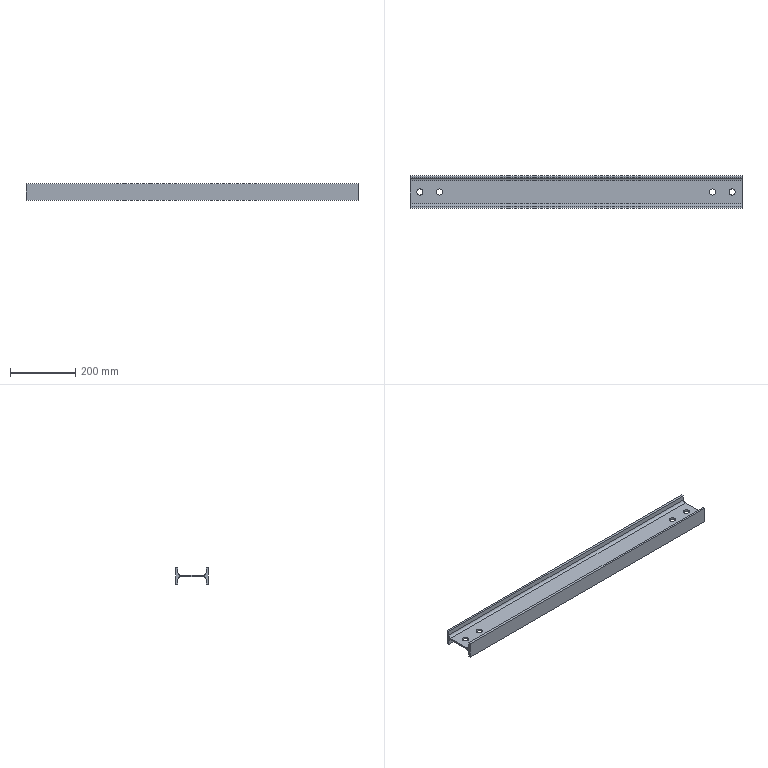Part | STEP file | Metering secondary beam 3 body_Default<As Machined> | 1 solid | 26 faces | box 1015 x 100 x 50 mm | volume 1197042 mm3 | plane 14 | cylinder 12 | commonest cylinder face diameters 19 x8 16 x4